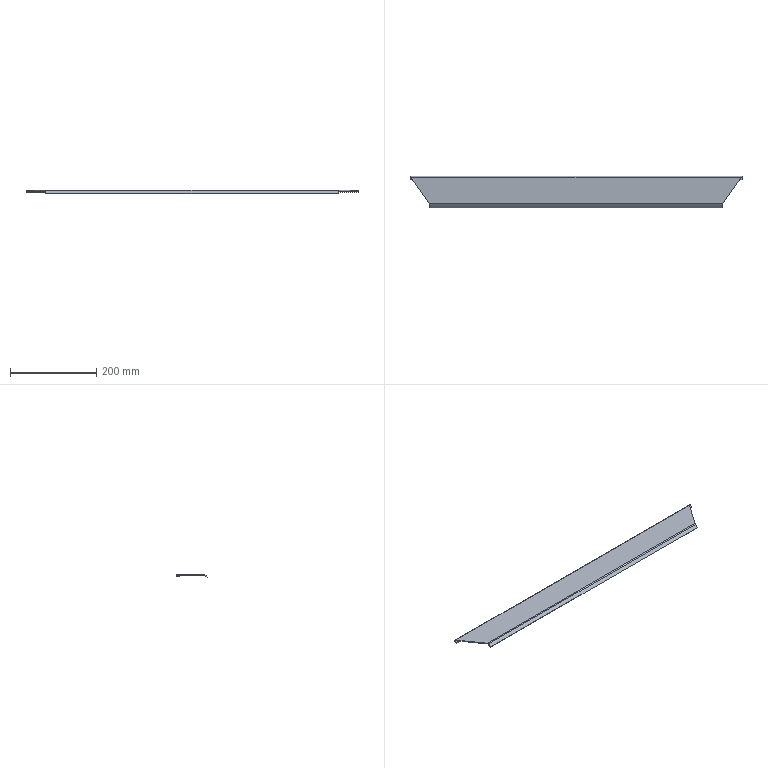Part | SolidWorks | features BaseBody 1 | 1 solid | 24 faces | box 772 x 72.66 x 7.96 mm | volume 118787 mm3 | plane 16 | cylinder 6 | spline 2 | commonest cylinder face diameters 1 x2 5 x2 4 x1 8 x1
STEP:
#1=CARTESIAN_POINT('',(-386.,30.,-3.));
#2=VERTEX_POINT('',#1);
#3=CARTESIAN_POINT('',(-386.,32.5,-0.5));
#4=VERTEX_POINT('',#3);
#5=CARTESIAN_POINT('',(-386.,30.,-0.5));
#6=DIRECTION('',(1.,0.,0.));
#7=DIRECTION('',(0.,1.,0.));
#8=AXIS2_PLACEMENT_3D('',#5,#6,#7);
#9=CIRCLE('',#8,2.5);
#10=EDGE_CURVE('',#2,#4,#9,.T.);
#11=ORIENTED_EDGE('',*,*,#10,.T.);
#12=CARTESIAN_POINT('',(386.,32.5,-0.5));
#13=VERTEX_POINT('',#12);
#14=CARTESIAN_POINT('',(-386.,32.5,-0.5));
#15=DIRECTION('',(1.,0.,0.));
#16=VECTOR('',#15,1000.);
#17=LINE('',#14,#16);
#18=EDGE_CURVE('',#4,#13,#17,.T.);
#19=ORIENTED_EDGE('',*,*,#18,.T.);
#20=CARTESIAN_POINT('',(386.,30.,-3.));
#21=VERTEX_POINT('',#20);
#22=CARTESIAN_POINT('',(386.,30.,-0.5));
#23=DIRECTION('',(-1.,0.,0.));
#24=DIRECTION('',(0.,1.,0.));
#25=AXIS2_PLACEMENT_3D('',#22,#23,#24);
#26=CIRCLE('',#25,2.5);
#27=EDGE_CURVE('',#13,#21,#26,.T.);
#28=ORIENTED_EDGE('',*,*,#27,.T.);
#29=CARTESIAN_POINT('',(-386.,30.,-3.));
#30=DIRECTION('',(-1.,0.,0.));
#31=VECTOR('',#30,1000.);
#32=LINE('',#29,#31);
#33=EDGE_CURVE('',#21,#2,#32,.T.);
#34=ORIENTED_EDGE('',*,*,#33,.T.);
#35=EDGE_LOOP('',(#11,#19,#28,#34));
#36=FACE_OUTER_BOUND('',#35,.T.);
#37=CARTESIAN_POINT('',(-386.,30.,-0.5));
#38=DIRECTION('',(1.,0.,0.));
#39=DIRECTION('',(0.,1.,0.));
#40=AXIS2_PLACEMENT_3D('',#37,#38,#39);
#41=CYLINDRICAL_SURFACE('',#40,2.5);
#42=ADVANCED_FACE('',(#36),#41,.T.);
#43=CARTESIAN_POINT('',(-386.,30.,0.));
#44=VERTEX_POINT('',#43);
#45=CARTESIAN_POINT('',(-386.,30.5,-0.5));
#46=VERTEX_POINT('',#45);
#47=CARTESIAN_POINT('',(-386.,30.,-0.5));
#48=DIRECTION('',(-1.,0.,0.));
#49=DIRECTION('',(0.,1.,0.));
#50=AXIS2_PLACEMENT_3D('',#47,#48,#49);
#51=CIRCLE('',#50,0.5);
#52=EDGE_CURVE('',#44,#46,#51,.T.);
#53=ORIENTED_EDGE('',*,*,#52,.T.);
#54=CARTESIAN_POINT('',(386.,30.5,-0.5));
#55=VERTEX_POINT('',#54);
#56=CARTESIAN_POINT('',(-386.,30.5,-0.5));
#57=DIRECTION('',(1.,0.,0.));
#58=VECTOR('',#57,1000.);
#59=LINE('',#56,#58);
#60=EDGE_CURVE('',#46,#55,#59,.T.);
#61=ORIENTED_EDGE('',*,*,#60,.T.);
#62=CARTESIAN_POINT('',(386.,30.,0.));
#63=VERTEX_POINT('',#62);
#64=CARTESIAN_POINT('',(386.,30.,-0.5));
#65=DIRECTION('',(-1.,0.,0.));
#66=DIRECTION('',(0.,1.,0.));
#67=AXIS2_PLACEMENT_3D('',#64,#65,#66);
#68=CIRCLE('',#67,0.5);
#69=EDGE_CURVE('',#63,#55,#68,.T.);
#70=ORIENTED_EDGE('',*,*,#69,.F.);
#71=CARTESIAN_POINT('',(384.231,30.,0.));
#72=VERTEX_POINT('',#71);
#73=CARTESIAN_POINT('',(-386.,30.,0.));
#74=DIRECTION('',(1.,0.,0.));
#75=VECTOR('',#74,1000.);
#76=LINE('',#73,#75);
#77=EDGE_CURVE('',#72,#63,#76,.T.);
#78=ORIENTED_EDGE('',*,*,#77,.F.);
#79=CARTESIAN_POINT('',(-384.231,30.,0.));
#80=VERTEX_POINT('',#79);
#81=CARTESIAN_POINT('',(0.,30.,0.));
#82=DIRECTION('',(-1.,0.,0.));
#83=VECTOR('',#82,1000.);
#84=LINE('',#81,#83);
#85=EDGE_CURVE('',#72,#80,#84,.T.);
#86=ORIENTED_EDGE('',*,*,#85,.T.);
#87=CARTESIAN_POINT('',(-386.,30.,0.));
#88=DIRECTION('',(1.,0.,0.));
#89=VECTOR('',#88,1000.);
#90=LINE('',#87,#89);
#91=EDGE_CURVE('',#44,#80,#90,.T.);
#92=ORIENTED_EDGE('',*,*,#91,.F.);
#93=EDGE_LOOP('',(#53,#61,#70,#78,#86,#92));
#94=FACE_OUTER_BOUND('',#93,.T.);
#95=CARTESIAN_POINT('',(-386.,30.,-0.5));
#96=DIRECTION('',(1.,0.,0.));
#97=DIRECTION('',(0.,1.,0.));
#98=AXIS2_PLACEMENT_3D('',#95,#96,#97);
#99=CYLINDRICAL_SURFACE('',#98,0.5);
#100=ADVANCED_FACE('',(#94),#99,.F.);
#101=CARTESIAN_POINT('',(-341.03,-31.044,2.));
#102=VERTEX_POINT('',#101);
#103=CARTESIAN_POINT('',(341.03,-31.044,2.));
#104=VERTEX_POINT('',#103);
#105=CARTESIAN_POINT('',(0.,-31.044,2.));
#106=DIRECTION('',(1.,0.,0.));
#107=VECTOR('',#106,1000.);
#108=LINE('',#105,#107);
#109=EDGE_CURVE('',#102,#104,#108,.T.);
#110=ORIENTED_EDGE('',*,*,#109,.T.);
#111=CARTESIAN_POINT('',(384.231,30.,2.));
#112=VERTEX_POINT('',#111);
#113=CARTESIAN_POINT('',(341.03,-31.044,2.));
#114=DIRECTION('',(0.5777,0.8163,0.));
#115=VECTOR('',#114,1000.);
#116=LINE('',#113,#115);
#117=EDGE_CURVE('',#104,#112,#116,.T.);
#118=ORIENTED_EDGE('',*,*,#117,.T.);
#119=CARTESIAN_POINT('',(-384.231,30.,2.));
#120=VERTEX_POINT('',#119);
#121=CARTESIAN_POINT('',(0.,30.,2.));
#122=DIRECTION('',(-1.,0.,0.));
#123=VECTOR('',#122,1000.);
#124=LINE('',#121,#123);
#125=EDGE_CURVE('',#112,#120,#124,.T.);
#126=ORIENTED_EDGE('',*,*,#125,.T.);
#127=CARTESIAN_POINT('',(-384.231,30.,2.));
#128=DIRECTION('',(0.5777,-0.8163,0.));
#129=VECTOR('',#128,1000.);
#130=LINE('',#127,#129);
#131=EDGE_CURVE('',#120,#102,#130,.T.);
#132=ORIENTED_EDGE('',*,*,#131,.T.);
#133=EDGE_LOOP('',(#110,#118,#126,#132));
#134=FACE_OUTER_BOUND('',#133,.T.);
#135=CARTESIAN_POINT('',(0.,1.856,2.));
#136=DIRECTION('',(0.,0.,1.));
#137=DIRECTION('',(1.,0.,0.));
#138=AXIS2_PLACEMENT_3D('',#135,#136,#137);
#139=PLANE('',#138);
#140=ADVANCED_FACE('',(#134),#139,.T.);
#141=CARTESIAN_POINT('',(341.03,-31.044,0.));
#142=VERTEX_POINT('',#141);
#143=CARTESIAN_POINT('',(341.03,-31.044,0.));
#144=DIRECTION('',(0.,0.,-1.));
#145=VECTOR('',#144,1000.);
#146=LINE('',#143,#145);
#147=EDGE_CURVE('',#104,#142,#146,.T.);
#148=ORIENTED_EDGE('',*,*,#147,.T.);
#149=CARTESIAN_POINT('',(386.,32.5,0.));
#150=DIRECTION('',(0.5777,0.8163,0.));
#151=VECTOR('',#150,1000.);
#152=LINE('',#149,#151);
#153=EDGE_CURVE('',#142,#72,#152,.T.);
#154=ORIENTED_EDGE('',*,*,#153,.T.);
#155=CARTESIAN_POINT('',(384.231,30.,0.));
#156=DIRECTION('',(0.,0.,1.));
#157=VECTOR('',#156,1000.);
#158=LINE('',#155,#157);
#159=EDGE_CURVE('',#72,#112,#158,.T.);
#160=ORIENTED_EDGE('',*,*,#159,.T.);
#161=ORIENTED_EDGE('',*,*,#117,.F.);
#162=EDGE_LOOP('',(#148,#154,#160,#161));
#163=FACE_OUTER_BOUND('',#162,.T.);
#164=CARTESIAN_POINT('',(386.,32.5,0.));
#165=DIRECTION('',(0.8163,-0.5777,0.));
#166=DIRECTION('',(0.5777,0.8163,0.));
#167=AXIS2_PLACEMENT_3D('',#164,#165,#166);
#168=PLANE('',#167);
#169=ADVANCED_FACE('',(#163),#168,.T.);
#170=ORIENTED_EDGE('',*,*,#109,.F.);
#171=CARTESIAN_POINT('',(-340.,-33.615,1.064));
#172=VERTEX_POINT('',#171);
#173=CARTESIAN_POINT('',(-341.03,-31.044,2.));
#174=CARTESIAN_POINT('',(-340.858,-31.512,2.));
#175=CARTESIAN_POINT('',(-340.686,-31.977,1.918));
#176=CARTESIAN_POINT('',(-340.341,-32.856,1.597));
#177=CARTESIAN_POINT('',(-340.173,-33.257,1.365));
#178=CARTESIAN_POINT('',(-340.,-33.615,1.064));
#179=B_SPLINE_CURVE_WITH_KNOTS('',3,(#173,#174,#175,#176,#177,#178),.UNSPECIFIED.,.F.,.F.,(4,2,4),(0.,0.001491,0.002983),.UNSPECIFIED.);
#180=EDGE_CURVE('',#102,#172,#179,.T.);
#181=ORIENTED_EDGE('',*,*,#180,.T.);
#182=CARTESIAN_POINT('',(340.,-33.615,1.064));
#183=VERTEX_POINT('',#182);
#184=CARTESIAN_POINT('',(0.,-33.615,1.064));
#185=DIRECTION('',(1.,0.,0.));
#186=VECTOR('',#185,1000.);
#187=LINE('',#184,#186);
#188=EDGE_CURVE('',#172,#183,#187,.T.);
#189=ORIENTED_EDGE('',*,*,#188,.T.);
#190=CARTESIAN_POINT('',(340.,-33.615,1.064));
#191=CARTESIAN_POINT('',(340.173,-33.257,1.365));
#192=CARTESIAN_POINT('',(340.344,-32.848,1.601));
#193=CARTESIAN_POINT('',(340.689,-31.968,1.92));
#194=CARTESIAN_POINT('',(340.858,-31.512,2.));
#195=CARTESIAN_POINT('',(341.03,-31.044,2.));
#196=B_SPLINE_CURVE_WITH_KNOTS('',3,(#190,#191,#192,#193,#194,#195),.UNSPECIFIED.,.F.,.F.,(4,2,4),(0.,0.001491,0.002983),.UNSPECIFIED.);
#197=EDGE_CURVE('',#183,#104,#196,.T.);
#198=ORIENTED_EDGE('',*,*,#197,.T.);
#199=EDGE_LOOP('',(#170,#181,#189,#198));
#200=FACE_OUTER_BOUND('',#199,.T.);
#201=CARTESIAN_POINT('',(0.,-31.044,-2.));
#202=DIRECTION('',(1.,0.,0.));
#203=DIRECTION('',(0.,1.,0.));
#204=AXIS2_PLACEMENT_3D('',#201,#202,#203);
#205=CYLINDRICAL_SURFACE('',#204,4.);
#206=ADVANCED_FACE('',(#200),#205,.T.);
#207=CARTESIAN_POINT('',(-341.03,-31.044,0.));
#208=VERTEX_POINT('',#207);
#209=CARTESIAN_POINT('',(-341.03,-31.044,0.));
#210=DIRECTION('',(0.,0.,1.));
#211=VECTOR('',#210,1000.);
#212=LINE('',#209,#211);
#213=EDGE_CURVE('',#208,#102,#212,.T.);
#214=ORIENTED_EDGE('',*,*,#213,.T.);
#215=ORIENTED_EDGE('',*,*,#131,.F.);
#216=CARTESIAN_POINT('',(-384.231,30.,0.));
#217=DIRECTION('',(0.,0.,-1.));
#218=VECTOR('',#217,1000.);
#219=LINE('',#216,#218);
#220=EDGE_CURVE('',#120,#80,#219,.T.);
#221=ORIENTED_EDGE('',*,*,#220,.T.);
#222=CARTESIAN_POINT('',(-340.,-32.5,0.));
#223=DIRECTION('',(0.5777,-0.8163,0.));
#224=VECTOR('',#223,1000.);
#225=LINE('',#222,#224);
#226=EDGE_CURVE('',#80,#208,#225,.T.);
#227=ORIENTED_EDGE('',*,*,#226,.T.);
#228=EDGE_LOOP('',(#214,#215,#221,#227));
#229=FACE_OUTER_BOUND('',#228,.T.);
#230=CARTESIAN_POINT('',(-340.,-32.5,0.));
#231=DIRECTION('',(-0.8163,-0.5777,0.));
#232=DIRECTION('',(0.5777,-0.8163,0.));
#233=AXIS2_PLACEMENT_3D('',#230,#231,#232);
#234=PLANE('',#233);
#235=ADVANCED_FACE('',(#229),#234,.T.);
#236=ORIENTED_EDGE('',*,*,#18,.F.);
#237=CARTESIAN_POINT('',(-386.,30.,2.));
#238=VERTEX_POINT('',#237);
#239=CARTESIAN_POINT('',(-386.,30.,-0.5));
#240=DIRECTION('',(1.,0.,0.));
#241=DIRECTION('',(0.,1.,0.));
#242=AXIS2_PLACEMENT_3D('',#239,#240,#241);
#243=CIRCLE('',#242,2.5);
#244=EDGE_CURVE('',#4,#238,#243,.T.);
#245=ORIENTED_EDGE('',*,*,#244,.T.);
#246=CARTESIAN_POINT('',(-386.,30.,2.));
#247=DIRECTION('',(1.,0.,0.));
#248=VECTOR('',#247,1000.);
#249=LINE('',#246,#248);
#250=EDGE_CURVE('',#238,#120,#249,.T.);
#251=ORIENTED_EDGE('',*,*,#250,.T.);
#252=ORIENTED_EDGE('',*,*,#125,.F.);
#253=CARTESIAN_POINT('',(386.,30.,2.));
#254=VERTEX_POINT('',#253);
#255=CARTESIAN_POINT('',(-386.,30.,2.));
#256=DIRECTION('',(1.,0.,0.));
#257=VECTOR('',#256,1000.);
#258=LINE('',#255,#257);
#259=EDGE_CURVE('',#112,#254,#258,.T.);
#260=ORIENTED_EDGE('',*,*,#259,.T.);
#261=CARTESIAN_POINT('',(386.,30.,-0.5));
#262=DIRECTION('',(-1.,0.,0.));
#263=DIRECTION('',(0.,1.,0.));
#264=AXIS2_PLACEMENT_3D('',#261,#262,#263);
#265=CIRCLE('',#264,2.5);
#266=EDGE_CURVE('',#254,#13,#265,.T.);
#267=ORIENTED_EDGE('',*,*,#266,.T.);
#268=EDGE_LOOP('',(#236,#245,#251,#252,#260,#267));
#269=FACE_OUTER_BOUND('',#268,.T.);
#270=CARTESIAN_POINT('',(-386.,30.,-0.5));
#271=DIRECTION('',(1.,0.,0.));
#272=DIRECTION('',(0.,1.,0.));
#273=AXIS2_PLACEMENT_3D('',#270,#271,#272);
#274=CYLINDRICAL_SURFACE('',#273,2.5);
#275=ADVANCED_FACE('',(#269),#274,.T.);
#276=ORIENTED_EDGE('',*,*,#153,.F.);
#277=CARTESIAN_POINT('',(0.,-31.044,0.));
#278=DIRECTION('',(1.,0.,0.));
#279=VECTOR('',#278,1000.);
#280=LINE('',#277,#279);
#281=EDGE_CURVE('',#208,#142,#280,.T.);
#282=ORIENTED_EDGE('',*,*,#281,.F.);
#283=ORIENTED_EDGE('',*,*,#226,.F.);
#284=ORIENTED_EDGE('',*,*,#85,.F.);
#285=EDGE_LOOP('',(#276,#282,#283,#284));
#286=FACE_OUTER_BOUND('',#285,.T.);
#287=CARTESIAN_POINT('',(0.,1.856,0.));
#288=DIRECTION('',(0.,0.,1.));
#289=DIRECTION('',(1.,0.,0.));
#290=AXIS2_PLACEMENT_3D('',#287,#288,#289);
#291=PLANE('',#290);
#292=ADVANCED_FACE('',(#286),#291,.F.);
#293=ORIENTED_EDGE('',*,*,#197,.F.);
#294=CARTESIAN_POINT('',(340.,-32.33,-0.4679));
#295=VERTEX_POINT('',#294);
#296=CARTESIAN_POINT('',(340.,-32.972,0.2981));
#297=DIRECTION('',(0.,0.6428,-0.766));
#298=VECTOR('',#297,1000.);
#299=LINE('',#296,#298);
#300=EDGE_CURVE('',#183,#295,#299,.T.);
#301=ORIENTED_EDGE('',*,*,#300,.T.);
#302=CARTESIAN_POINT('',(340.,-32.33,-0.4679));
#303=CARTESIAN_POINT('',(340.172,-32.151,-0.3178));
#304=CARTESIAN_POINT('',(340.344,-31.946,-0.2));
#305=CARTESIAN_POINT('',(340.687,-31.509,-0.04081));
#306=CARTESIAN_POINT('',(340.858,-31.278,0.));
#307=CARTESIAN_POINT('',(341.03,-31.044,0.));
#308=B_SPLINE_CURVE_WITH_KNOTS('',3,(#302,#303,#304,#305,#306,#307),.UNSPECIFIED.,.F.,.F.,(4,2,4),(0.,0.0008676,0.001735),.UNSPECIFIED.);
#309=EDGE_CURVE('',#295,#142,#308,.T.);
#310=ORIENTED_EDGE('',*,*,#309,.T.);
#311=ORIENTED_EDGE('',*,*,#147,.F.);
#312=EDGE_LOOP('',(#293,#301,#310,#311));
#313=FACE_OUTER_BOUND('',#312,.T.);
#314=CARTESIAN_POINT('',(340.,-33.628,1.079));
#315=CARTESIAN_POINT('',(340.343,-32.911,1.681));
#316=CARTESIAN_POINT('',(340.687,-31.98,2.02));
#317=CARTESIAN_POINT('',(341.03,-31.044,2.02));
#318=CARTESIAN_POINT('',(340.,-33.624,1.074));
#319=CARTESIAN_POINT('',(340.343,-32.908,1.675));
#320=CARTESIAN_POINT('',(340.687,-31.978,2.013));
#321=CARTESIAN_POINT('',(341.03,-31.044,2.013));
#322=CARTESIAN_POINT('',(340.,-33.62,1.069));
#323=CARTESIAN_POINT('',(340.343,-32.905,1.669));
#324=CARTESIAN_POINT('',(340.687,-31.977,2.007));
#325=CARTESIAN_POINT('',(341.03,-31.044,2.007));
#326=CARTESIAN_POINT('',(340.,-33.615,1.064));
#327=CARTESIAN_POINT('',(340.343,-32.902,1.663));
#328=CARTESIAN_POINT('',(340.687,-31.975,2.));
#329=CARTESIAN_POINT('',(341.03,-31.044,2.));
#330=CARTESIAN_POINT('',(340.,-33.187,0.5535));
#331=CARTESIAN_POINT('',(340.343,-32.593,1.052));
#332=CARTESIAN_POINT('',(340.687,-31.82,1.333));
#333=CARTESIAN_POINT('',(341.03,-31.044,1.333));
#334=CARTESIAN_POINT('',(340.,-32.758,0.04279));
#335=CARTESIAN_POINT('',(340.343,-32.283,0.4417));
#336=CARTESIAN_POINT('',(340.687,-31.665,0.6667));
#337=CARTESIAN_POINT('',(341.03,-31.044,0.6667));
#338=CARTESIAN_POINT('',(340.,-32.33,-0.4679));
#339=CARTESIAN_POINT('',(340.343,-31.973,-0.1687));
#340=CARTESIAN_POINT('',(340.687,-31.51,0.));
#341=CARTESIAN_POINT('',(341.03,-31.044,0.));
#342=B_SPLINE_SURFACE_WITH_KNOTS('',3,3,((#314,#315,#316,#317),(#318,#319,#320,#321),(#322,#323,#324,#325),(#326,#327,#328,#329),(#330,#331,#332,#333),(#334,#335,#336,#337),(#338,#339,#340,#341)),.UNSPECIFIED.,.F.,.F.,.F.,(4,3,4),(4,4),(-0.002,0.,0.2),(0.,0.2259),.UNSPECIFIED.);
#343=ADVANCED_FACE('',(#313),#342,.T.);
#344=CARTESIAN_POINT('',(386.,30.,0.));
#345=DIRECTION('',(0.,0.,1.));
#346=VECTOR('',#345,1000.);
#347=LINE('',#344,#346);
#348=EDGE_CURVE('',#63,#254,#347,.T.);
#349=ORIENTED_EDGE('',*,*,#348,.T.);
#350=ORIENTED_EDGE('',*,*,#259,.F.);
#351=ORIENTED_EDGE('',*,*,#159,.F.);
#352=ORIENTED_EDGE('',*,*,#77,.T.);
#353=EDGE_LOOP('',(#349,#350,#351,#352));
#354=FACE_OUTER_BOUND('',#353,.T.);
#355=CARTESIAN_POINT('',(-386.,30.,0.));
#356=DIRECTION('',(0.,-1.,0.));
#357=DIRECTION('',(0.,0.,-1.));
#358=AXIS2_PLACEMENT_3D('',#355,#356,#357);
#359=PLANE('',#358);
#360=ADVANCED_FACE('',(#354),#359,.T.);
#361=ORIENTED_EDGE('',*,*,#213,.F.);
#362=CARTESIAN_POINT('',(-340.,-32.33,-0.4679));
#363=VERTEX_POINT('',#362);
#364=CARTESIAN_POINT('',(-341.03,-31.044,0.));
#365=CARTESIAN_POINT('',(-340.858,-31.278,0.));
#366=CARTESIAN_POINT('',(-340.686,-31.51,-0.04111));
#367=CARTESIAN_POINT('',(-340.343,-31.948,-0.2006));
#368=CARTESIAN_POINT('',(-340.172,-32.151,-0.3178));
#369=CARTESIAN_POINT('',(-340.,-32.33,-0.4679));
#370=B_SPLINE_CURVE_WITH_KNOTS('',3,(#364,#365,#366,#367,#368,#369),.UNSPECIFIED.,.F.,.F.,(4,2,4),(0.,0.0008676,0.001735),.UNSPECIFIED.);
#371=EDGE_CURVE('',#208,#363,#370,.T.);
#372=ORIENTED_EDGE('',*,*,#371,.T.);
#373=CARTESIAN_POINT('',(-340.,-32.972,0.2981));
#374=DIRECTION('',(0.,-0.6428,0.766));
#375=VECTOR('',#374,1000.);
#376=LINE('',#373,#375);
#377=EDGE_CURVE('',#363,#172,#376,.T.);
#378=ORIENTED_EDGE('',*,*,#377,.T.);
#379=ORIENTED_EDGE('',*,*,#180,.F.);
#380=EDGE_LOOP('',(#361,#372,#378,#379));
#381=FACE_OUTER_BOUND('',#380,.T.);
#382=CARTESIAN_POINT('',(-340.,-32.33,-0.4679));
#383=CARTESIAN_POINT('',(-340.343,-31.973,-0.1687));
#384=CARTESIAN_POINT('',(-340.687,-31.51,0.));
#385=CARTESIAN_POINT('',(-341.03,-31.044,0.));
#386=CARTESIAN_POINT('',(-340.,-32.758,0.04279));
#387=CARTESIAN_POINT('',(-340.343,-32.283,0.4417));
#388=CARTESIAN_POINT('',(-340.687,-31.665,0.6667));
#389=CARTESIAN_POINT('',(-341.03,-31.044,0.6667));
#390=CARTESIAN_POINT('',(-340.,-33.187,0.5535));
#391=CARTESIAN_POINT('',(-340.343,-32.593,1.052));
#392=CARTESIAN_POINT('',(-340.687,-31.82,1.333));
#393=CARTESIAN_POINT('',(-341.03,-31.044,1.333));
#394=CARTESIAN_POINT('',(-340.,-33.615,1.064));
#395=CARTESIAN_POINT('',(-340.343,-32.902,1.663));
#396=CARTESIAN_POINT('',(-340.687,-31.975,2.));
#397=CARTESIAN_POINT('',(-341.03,-31.044,2.));
#398=CARTESIAN_POINT('',(-340.,-33.62,1.069));
#399=CARTESIAN_POINT('',(-340.343,-32.905,1.669));
#400=CARTESIAN_POINT('',(-340.687,-31.977,2.007));
#401=CARTESIAN_POINT('',(-341.03,-31.044,2.007));
#402=CARTESIAN_POINT('',(-340.,-33.624,1.074));
#403=CARTESIAN_POINT('',(-340.343,-32.908,1.675));
#404=CARTESIAN_POINT('',(-340.687,-31.978,2.013));
#405=CARTESIAN_POINT('',(-341.03,-31.044,2.013));
#406=CARTESIAN_POINT('',(-340.,-33.628,1.079));
#407=CARTESIAN_POINT('',(-340.343,-32.911,1.681));
#408=CARTESIAN_POINT('',(-340.687,-31.98,2.02));
#409=CARTESIAN_POINT('',(-341.03,-31.044,2.02));
#410=B_SPLINE_SURFACE_WITH_KNOTS('',3,3,((#382,#383,#384,#385),(#386,#387,#388,#389),(#390,#391,#392,#393),(#394,#395,#396,#397),(#398,#399,#400,#401),(#402,#403,#404,#405),(#406,#407,#408,#409)),.UNSPECIFIED.,.F.,.F.,.F.,(4,3,4),(4,4),(-0.2,0.,0.002),(-0.2259,0.),.UNSPECIFIED.);
#411=ADVANCED_FACE('',(#381),#410,.T.);
#412=CARTESIAN_POINT('',(-340.,-40.16,-4.428));
#413=VERTEX_POINT('',#412);
#414=CARTESIAN_POINT('',(340.,-40.16,-4.428));
#415=VERTEX_POINT('',#414);
#416=CARTESIAN_POINT('',(0.,-40.16,-4.428));
#417=DIRECTION('',(1.,0.,0.));
#418=VECTOR('',#417,1000.);
#419=LINE('',#416,#418);
#420=EDGE_CURVE('',#413,#415,#419,.T.);
#421=ORIENTED_EDGE('',*,*,#420,.T.);
#422=CARTESIAN_POINT('',(340.,-36.111,-1.03));
#423=DIRECTION('',(0.,0.766,0.6428));
#424=VECTOR('',#423,1000.);
#425=LINE('',#422,#424);
#426=EDGE_CURVE('',#415,#183,#425,.T.);
#427=ORIENTED_EDGE('',*,*,#426,.T.);
#428=ORIENTED_EDGE('',*,*,#188,.F.);
#429=CARTESIAN_POINT('',(-340.,-36.111,-1.03));
#430=DIRECTION('',(0.,-0.766,-0.6428));
#431=VECTOR('',#430,1000.);
#432=LINE('',#429,#431);
#433=EDGE_CURVE('',#172,#413,#432,.T.);
#434=ORIENTED_EDGE('',*,*,#433,.T.);
#435=EDGE_LOOP('',(#421,#427,#428,#434));
#436=FACE_OUTER_BOUND('',#435,.T.);
#437=CARTESIAN_POINT('',(0.,-36.111,-1.03));
#438=DIRECTION('',(0.,-0.6428,0.766));
#439=DIRECTION('',(0.,-0.766,-0.6428));
#440=AXIS2_PLACEMENT_3D('',#437,#438,#439);
#441=PLANE('',#440);
#442=ADVANCED_FACE('',(#436),#441,.T.);
#443=CARTESIAN_POINT('',(-386.,30.,0.));
#444=DIRECTION('',(0.,0.,-1.));
#445=VECTOR('',#444,1000.);
#446=LINE('',#443,#445);
#447=EDGE_CURVE('',#238,#44,#446,.T.);
#448=ORIENTED_EDGE('',*,*,#447,.T.);
#449=ORIENTED_EDGE('',*,*,#91,.T.);
#450=ORIENTED_EDGE('',*,*,#220,.F.);
#451=ORIENTED_EDGE('',*,*,#250,.F.);
#452=EDGE_LOOP('',(#448,#449,#450,#451));
#453=FACE_OUTER_BOUND('',#452,.T.);
#454=CARTESIAN_POINT('',(-386.,30.,0.));
#455=DIRECTION('',(0.,-1.,0.));
#456=DIRECTION('',(0.,0.,-1.));
#457=AXIS2_PLACEMENT_3D('',#454,#455,#456);
#458=PLANE('',#457);
#459=ADVANCED_FACE('',(#453),#458,.T.);
#460=ORIENTED_EDGE('',*,*,#52,.F.);
#461=ORIENTED_EDGE('',*,*,#447,.F.);
#462=ORIENTED_EDGE('',*,*,#244,.F.);
#463=ORIENTED_EDGE('',*,*,#10,.F.);
#464=CARTESIAN_POINT('',(-386.,24.5,-3.));
#465=VERTEX_POINT('',#464);
#466=CARTESIAN_POINT('',(-386.,30.,-3.));
#467=DIRECTION('',(0.,1.,0.));
#468=VECTOR('',#467,1000.);
#469=LINE('',#466,#468);
#470=EDGE_CURVE('',#465,#2,#469,.T.);
#471=ORIENTED_EDGE('',*,*,#470,.F.);
#472=CARTESIAN_POINT('',(-386.,24.5,-1.));
#473=VERTEX_POINT('',#472);
#474=CARTESIAN_POINT('',(-386.,24.5,-1.176));
#475=DIRECTION('',(0.,0.,-1.));
#476=VECTOR('',#475,1000.);
#477=LINE('',#474,#476);
#478=EDGE_CURVE('',#473,#465,#477,.T.);
#479=ORIENTED_EDGE('',*,*,#478,.F.);
#480=CARTESIAN_POINT('',(-386.,30.,-1.));
#481=VERTEX_POINT('',#480);
#482=CARTESIAN_POINT('',(-386.,28.791,-1.));
#483=DIRECTION('',(0.,-1.,0.));
#484=VECTOR('',#483,1000.);
#485=LINE('',#482,#484);
#486=EDGE_CURVE('',#481,#473,#485,.T.);
#487=ORIENTED_EDGE('',*,*,#486,.F.);
#488=CARTESIAN_POINT('',(-386.,30.,-0.5));
#489=DIRECTION('',(-1.,0.,0.));
#490=DIRECTION('',(0.,1.,0.));
#491=AXIS2_PLACEMENT_3D('',#488,#489,#490);
#492=CIRCLE('',#491,0.5);
#493=EDGE_CURVE('',#46,#481,#492,.T.);
#494=ORIENTED_EDGE('',*,*,#493,.F.);
#495=EDGE_LOOP('',(#460,#461,#462,#463,#471,#479,#487,#494));
#496=FACE_OUTER_BOUND('',#495,.T.);
#497=CARTESIAN_POINT('',(-386.,28.791,-1.176));
#498=DIRECTION('',(1.,0.,0.));
#499=DIRECTION('',(0.,0.,-1.));
#500=AXIS2_PLACEMENT_3D('',#497,#498,#499);
#501=PLANE('',#500);
#502=ADVANCED_FACE('',(#496),#501,.F.);
#503=ORIENTED_EDGE('',*,*,#470,.T.);
#504=ORIENTED_EDGE('',*,*,#33,.F.);
#505=CARTESIAN_POINT('',(386.,24.5,-3.));
#506=VERTEX_POINT('',#505);
#507=CARTESIAN_POINT('',(386.,30.,-3.));
#508=DIRECTION('',(0.,-1.,0.));
#509=VECTOR('',#508,1000.);
#510=LINE('',#507,#509);
#511=EDGE_CURVE('',#21,#506,#510,.T.);
#512=ORIENTED_EDGE('',*,*,#511,.T.);
#513=CARTESIAN_POINT('',(-386.,24.5,-3.));
#514=DIRECTION('',(-1.,0.,0.));
#515=VECTOR('',#514,1000.);
#516=LINE('',#513,#515);
#517=EDGE_CURVE('',#506,#465,#516,.T.);
#518=ORIENTED_EDGE('',*,*,#517,.T.);
#519=EDGE_LOOP('',(#503,#504,#512,#518));
#520=FACE_OUTER_BOUND('',#519,.T.);
#521=CARTESIAN_POINT('',(-386.,30.,-3.));
#522=DIRECTION('',(0.,0.,-1.));
#523=DIRECTION('',(0.,1.,0.));
#524=AXIS2_PLACEMENT_3D('',#521,#522,#523);
#525=PLANE('',#524);
#526=ADVANCED_FACE('',(#520),#525,.T.);
#527=ORIENTED_EDGE('',*,*,#348,.F.);
#528=ORIENTED_EDGE('',*,*,#69,.T.);
#529=CARTESIAN_POINT('',(386.,30.,-1.));
#530=VERTEX_POINT('',#529);
#531=CARTESIAN_POINT('',(386.,30.,-0.5));
#532=DIRECTION('',(-1.,0.,0.));
#533=DIRECTION('',(0.,1.,0.));
#534=AXIS2_PLACEMENT_3D('',#531,#532,#533);
#535=CIRCLE('',#534,0.5);
#536=EDGE_CURVE('',#55,#530,#535,.T.);
#537=ORIENTED_EDGE('',*,*,#536,.T.);
#538=CARTESIAN_POINT('',(386.,24.5,-1.));
#539=VERTEX_POINT('',#538);
#540=CARTESIAN_POINT('',(386.,28.791,-1.));
#541=DIRECTION('',(0.,-1.,0.));
#542=VECTOR('',#541,1000.);
#543=LINE('',#540,#542);
#544=EDGE_CURVE('',#530,#539,#543,.T.);
#545=ORIENTED_EDGE('',*,*,#544,.T.);
#546=CARTESIAN_POINT('',(386.,24.5,-3.));
#547=DIRECTION('',(0.,0.,1.));
#548=VECTOR('',#547,1000.);
#549=LINE('',#546,#548);
#550=EDGE_CURVE('',#506,#539,#549,.T.);
#551=ORIENTED_EDGE('',*,*,#550,.F.);
#552=ORIENTED_EDGE('',*,*,#511,.F.);
#553=ORIENTED_EDGE('',*,*,#27,.F.);
#554=ORIENTED_EDGE('',*,*,#266,.F.);
#555=EDGE_LOOP('',(#527,#528,#537,#545,#551,#552,#553,#554));
#556=FACE_OUTER_BOUND('',#555,.T.);
#557=CARTESIAN_POINT('',(386.,28.791,-1.176));
#558=DIRECTION('',(1.,0.,0.));
#559=DIRECTION('',(0.,0.,-1.));
#560=AXIS2_PLACEMENT_3D('',#557,#558,#559);
#561=PLANE('',#560);
#562=ADVANCED_FACE('',(#556),#561,.T.);
#563=ORIENTED_EDGE('',*,*,#60,.F.);
#564=ORIENTED_EDGE('',*,*,#493,.T.);
#565=CARTESIAN_POINT('',(-386.,30.,-1.));
#566=DIRECTION('',(-1.,0.,0.));
#567=VECTOR('',#566,1000.);
#568=LINE('',#565,#567);
#569=EDGE_CURVE('',#530,#481,#568,.T.);
#570=ORIENTED_EDGE('',*,*,#569,.F.);
#571=ORIENTED_EDGE('',*,*,#536,.F.);
#572=EDGE_LOOP('',(#563,#564,#570,#571));
#573=FACE_OUTER_BOUND('',#572,.T.);
#574=CARTESIAN_POINT('',(-386.,30.,-0.5));
#575=DIRECTION('',(1.,0.,0.));
#576=DIRECTION('',(0.,1.,0.));
#577=AXIS2_PLACEMENT_3D('',#574,#575,#576);
#578=CYLINDRICAL_SURFACE('',#577,0.5);
#579=ADVANCED_FACE('',(#573),#578,.F.);
#580=ORIENTED_EDGE('',*,*,#371,.F.);
#581=ORIENTED_EDGE('',*,*,#281,.T.);
#582=ORIENTED_EDGE('',*,*,#309,.F.);
#583=CARTESIAN_POINT('',(0.,-32.33,-0.4679));
#584=DIRECTION('',(1.,0.,0.));
#585=VECTOR('',#584,1000.);
#586=LINE('',#583,#585);
#587=EDGE_CURVE('',#363,#295,#586,.T.);
#588=ORIENTED_EDGE('',*,*,#587,.F.);
#589=EDGE_LOOP('',(#580,#581,#582,#588));
#590=FACE_OUTER_BOUND('',#589,.T.);
#591=CARTESIAN_POINT('',(0.,-31.044,-2.));
#592=DIRECTION('',(1.,0.,0.));
#593=DIRECTION('',(0.,1.,0.));
#594=AXIS2_PLACEMENT_3D('',#591,#592,#593);
#595=CYLINDRICAL_SURFACE('',#594,2.);
#596=ADVANCED_FACE('',(#590),#595,.F.);
#597=ORIENTED_EDGE('',*,*,#426,.F.);
#598=CARTESIAN_POINT('',(340.,-38.875,-5.96));
#599=VERTEX_POINT('',#598);
#600=CARTESIAN_POINT('',(340.,-40.16,-4.428));
#601=DIRECTION('',(0.,0.6428,-0.766));
#602=VECTOR('',#601,1000.);
#603=LINE('',#600,#602);
#604=EDGE_CURVE('',#415,#599,#603,.T.);
#605=ORIENTED_EDGE('',*,*,#604,.T.);
#606=CARTESIAN_POINT('',(340.,-38.875,-5.96));
#607=DIRECTION('',(0.,0.766,0.6428));
#608=VECTOR('',#607,1000.);
#609=LINE('',#606,#608);
#610=EDGE_CURVE('',#599,#295,#609,.T.);
#611=ORIENTED_EDGE('',*,*,#610,.T.);
#612=ORIENTED_EDGE('',*,*,#300,.F.);
#613=EDGE_LOOP('',(#597,#605,#611,#612));
#614=FACE_OUTER_BOUND('',#613,.T.);
#615=CARTESIAN_POINT('',(340.,-40.16,-4.428));
#616=DIRECTION('',(1.,0.,0.));
#617=DIRECTION('',(0.,0.,-1.));
#618=AXIS2_PLACEMENT_3D('',#615,#616,#617);
#619=PLANE('',#618);
#620=ADVANCED_FACE('',(#614),#619,.T.);
#621=ORIENTED_EDGE('',*,*,#433,.F.);
#622=ORIENTED_EDGE('',*,*,#377,.F.);
#623=CARTESIAN_POINT('',(-340.,-38.875,-5.96));
#624=VERTEX_POINT('',#623);
#625=CARTESIAN_POINT('',(-340.,-32.33,-0.4679));
#626=DIRECTION('',(0.,-0.766,-0.6428));
#627=VECTOR('',#626,1000.);
#628=LINE('',#625,#627);
#629=EDGE_CURVE('',#363,#624,#628,.T.);
#630=ORIENTED_EDGE('',*,*,#629,.T.);
#631=CARTESIAN_POINT('',(-340.,-38.875,-5.96));
#632=DIRECTION('',(0.,-0.6428,0.766));
#633=VECTOR('',#632,1000.);
#634=LINE('',#631,#633);
#635=EDGE_CURVE('',#624,#413,#634,.T.);
#636=ORIENTED_EDGE('',*,*,#635,.T.);
#637=EDGE_LOOP('',(#621,#622,#630,#636));
#638=FACE_OUTER_BOUND('',#637,.T.);
#639=CARTESIAN_POINT('',(-340.,-33.615,1.064));
#640=DIRECTION('',(-1.,0.,0.));
#641=DIRECTION('',(0.,0.,1.));
#642=AXIS2_PLACEMENT_3D('',#639,#640,#641);
#643=PLANE('',#642);
#644=ADVANCED_FACE('',(#638),#643,.T.);
#645=ORIENTED_EDGE('',*,*,#420,.F.);
#646=ORIENTED_EDGE('',*,*,#635,.F.);
#647=CARTESIAN_POINT('',(-340.,-38.875,-5.96));
#648=DIRECTION('',(1.,0.,0.));
#649=VECTOR('',#648,1000.);
#650=LINE('',#647,#649);
#651=EDGE_CURVE('',#624,#599,#650,.T.);
#652=ORIENTED_EDGE('',*,*,#651,.T.);
#653=ORIENTED_EDGE('',*,*,#604,.F.);
#654=EDGE_LOOP('',(#645,#646,#652,#653));
#655=FACE_OUTER_BOUND('',#654,.T.);
#656=CARTESIAN_POINT('',(-340.,-40.16,-4.428));
#657=DIRECTION('',(0.,-0.766,-0.6428));
#658=DIRECTION('',(0.,0.6428,-0.766));
#659=AXIS2_PLACEMENT_3D('',#656,#657,#658);
#660=PLANE('',#659);
#661=ADVANCED_FACE('',(#655),#660,.T.);
#662=ORIENTED_EDGE('',*,*,#478,.T.);
#663=ORIENTED_EDGE('',*,*,#517,.F.);
#664=ORIENTED_EDGE('',*,*,#550,.T.);
#665=CARTESIAN_POINT('',(-386.,24.5,-1.));
#666=DIRECTION('',(-1.,0.,0.));
#667=VECTOR('',#666,1000.);
#668=LINE('',#665,#667);
#669=EDGE_CURVE('',#539,#473,#668,.T.);
#670=ORIENTED_EDGE('',*,*,#669,.T.);
#671=EDGE_LOOP('',(#662,#663,#664,#670));
#672=FACE_OUTER_BOUND('',#671,.T.);
#673=CARTESIAN_POINT('',(-386.,24.5,-3.));
#674=DIRECTION('',(0.,-1.,0.));
#675=DIRECTION('',(1.,0.,0.));
#676=AXIS2_PLACEMENT_3D('',#673,#674,#675);
#677=PLANE('',#676);
#678=ADVANCED_FACE('',(#672),#677,.T.);
#679=ORIENTED_EDGE('',*,*,#486,.T.);
#680=ORIENTED_EDGE('',*,*,#669,.F.);
#681=ORIENTED_EDGE('',*,*,#544,.F.);
#682=ORIENTED_EDGE('',*,*,#569,.T.);
#683=EDGE_LOOP('',(#679,#680,#681,#682));
#684=FACE_OUTER_BOUND('',#683,.T.);
#685=CARTESIAN_POINT('',(-386.,24.5,-1.));
#686=DIRECTION('',(0.,0.,1.));
#687=DIRECTION('',(0.,-1.,0.));
#688=AXIS2_PLACEMENT_3D('',#685,#686,#687);
#689=PLANE('',#688);
#690=ADVANCED_FACE('',(#684),#689,.T.);
#691=ORIENTED_EDGE('',*,*,#610,.F.);
#692=ORIENTED_EDGE('',*,*,#651,.F.);
#693=ORIENTED_EDGE('',*,*,#629,.F.);
#694=ORIENTED_EDGE('',*,*,#587,.T.);
#695=EDGE_LOOP('',(#691,#692,#693,#694));
#696=FACE_OUTER_BOUND('',#695,.T.);
#697=CARTESIAN_POINT('',(0.,-34.825,-2.562));
#698=DIRECTION('',(0.,-0.6428,0.766));
#699=DIRECTION('',(0.,-0.766,-0.6428));
#700=AXIS2_PLACEMENT_3D('',#697,#698,#699);
#701=PLANE('',#700);
#702=ADVANCED_FACE('',(#696),#701,.F.);
#703=CLOSED_SHELL('',(#42,#100,#140,#169,#206,#235,#275,#292,#343,#360,#411,#442,#459,#502,#526,#562,#579,#596,#620,#644,#661,#678,#690,#702));
#704=MANIFOLD_SOLID_BREP('',#703);
#705=CARTESIAN_POINT('',(0.,0.,0.));
#706=DIRECTION('',(0.,0.,1.));
#707=DIRECTION('',(1.,0.,0.));
#708=AXIS2_PLACEMENT_3D('',#705,#706,#707);
#709=(LENGTH_UNIT()NAMED_UNIT(*)SI_UNIT(.MILLI.,.METRE.));
#710=UNCERTAINTY_MEASURE_WITH_UNIT(LENGTH_MEASURE(0.00001),#709,'','');
#711=(NAMED_UNIT(*)PLANE_ANGLE_UNIT()SI_UNIT($,.RADIAN.));
#712=(NAMED_UNIT(*)SI_UNIT($,.STERADIAN.)SOLID_ANGLE_UNIT());
#713=(GEOMETRIC_REPRESENTATION_CONTEXT(3)GLOBAL_UNCERTAINTY_ASSIGNED_CONTEXT((#710))GLOBAL_UNIT_ASSIGNED_CONTEXT((#709,#711,#712))REPRESENTATION_CONTEXT('',''));
#714=ADVANCED_BREP_SHAPE_REPRESENTATION('',(#704,#708),#713);